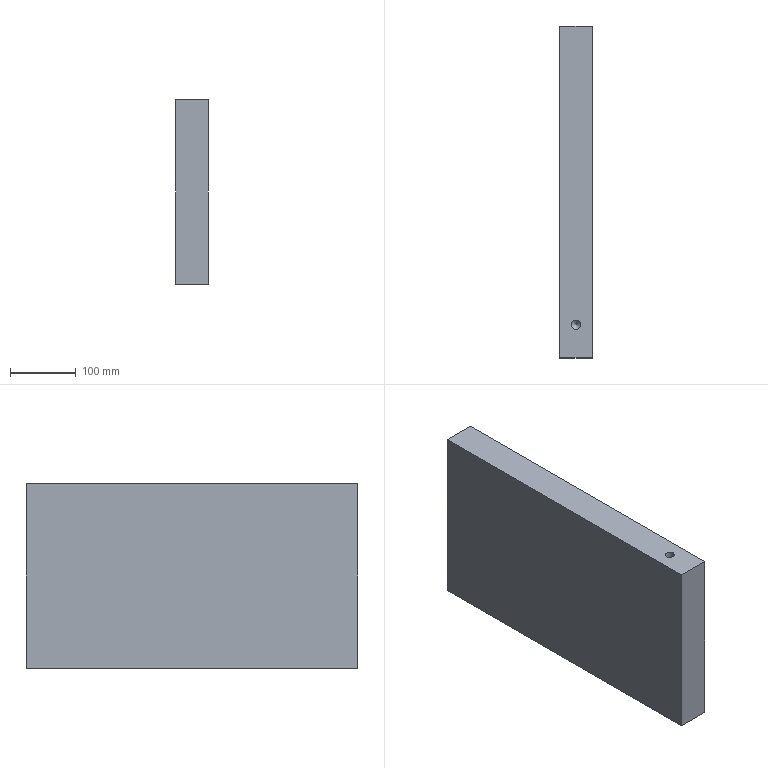Part | NX | features 29 2 | 1 solid | 12 faces | box 50 x 503.5 x 280.5 mm | volume 7043178 mm3 | plane 6 | cylinder 3 | cone 3 | commonest cylinder face diameters 14.1 x3
STEP:
#1=CARTESIAN_POINT('',(3262.05,-622.5,-493.5));
#2=VERTEX_POINT('',#1);
#3=CARTESIAN_POINT('',(3255.,-622.5,-493.5));
#4=DIRECTION('',(0.,0.,1.));
#5=DIRECTION('',(1.,0.,0.));
#6=AXIS2_PLACEMENT_3D('',#3,#4,#5);
#7=CIRCLE('',#6,7.05);
#8=EDGE_CURVE('',#2,#2,#7,.T.);
#9=ORIENTED_EDGE('',*,*,#8,.T.);
#10=EDGE_LOOP('',(#9));
#11=FACE_BOUND('',#10,.T.);
#12=CARTESIAN_POINT('',(3230.,-169.,-493.5));
#13=VERTEX_POINT('',#12);
#14=CARTESIAN_POINT('',(3230.,-672.5,-493.5));
#15=VERTEX_POINT('',#14);
#16=CARTESIAN_POINT('',(3230.,193.,-493.5));
#17=DIRECTION('',(0.,-1.,0.));
#18=VECTOR('',#17,1000.);
#19=LINE('',#16,#18);
#20=EDGE_CURVE('',#13,#15,#19,.T.);
#21=ORIENTED_EDGE('',*,*,#20,.F.);
#22=CARTESIAN_POINT('',(3280.,-169.,-493.5));
#23=VERTEX_POINT('',#22);
#24=CARTESIAN_POINT('',(1945.,-169.,-493.5));
#25=DIRECTION('',(1.,0.,0.));
#26=VECTOR('',#25,1000.);
#27=LINE('',#24,#26);
#28=EDGE_CURVE('',#13,#23,#27,.T.);
#29=ORIENTED_EDGE('',*,*,#28,.T.);
#30=CARTESIAN_POINT('',(3280.,-672.5,-493.5));
#31=VERTEX_POINT('',#30);
#32=CARTESIAN_POINT('',(3280.,193.,-493.5));
#33=DIRECTION('',(0.,1.,0.));
#34=VECTOR('',#33,1000.);
#35=LINE('',#32,#34);
#36=EDGE_CURVE('',#31,#23,#35,.T.);
#37=ORIENTED_EDGE('',*,*,#36,.F.);
#38=CARTESIAN_POINT('',(3620.,-672.5,-493.5));
#39=DIRECTION('',(-1.,0.,0.));
#40=VECTOR('',#39,1000.);
#41=LINE('',#38,#40);
#42=EDGE_CURVE('',#31,#15,#41,.T.);
#43=ORIENTED_EDGE('',*,*,#42,.T.);
#44=EDGE_LOOP('',(#21,#29,#37,#43));
#45=FACE_BOUND('',#44,.T.);
#46=CARTESIAN_POINT('',(3262.05,-242.5,-493.5));
#47=VERTEX_POINT('',#46);
#48=CARTESIAN_POINT('',(3255.,-242.5,-493.5));
#49=DIRECTION('',(0.,0.,1.));
#50=DIRECTION('',(1.,0.,0.));
#51=AXIS2_PLACEMENT_3D('',#48,#49,#50);
#52=CIRCLE('',#51,7.05);
#53=EDGE_CURVE('',#47,#47,#52,.T.);
#54=ORIENTED_EDGE('',*,*,#53,.T.);
#55=EDGE_LOOP('',(#54));
#56=FACE_BOUND('',#55,.T.);
#57=CARTESIAN_POINT('',(1945.,0.,-493.5));
#58=DIRECTION('',(0.,0.,-1.));
#59=DIRECTION('',(1.,0.,0.));
#60=AXIS2_PLACEMENT_3D('',#57,#58,#59);
#61=PLANE('',#60);
#62=ADVANCED_FACE('',(#11,#45,#56),#61,.T.);
#63=CARTESIAN_POINT('',(3280.,-169.,-213.));
#64=VERTEX_POINT('',#63);
#65=CARTESIAN_POINT('',(3280.,-672.5,-213.));
#66=VERTEX_POINT('',#65);
#67=CARTESIAN_POINT('',(3280.,193.,-213.));
#68=DIRECTION('',(0.,-1.,0.));
#69=VECTOR('',#68,1000.);
#70=LINE('',#67,#69);
#71=EDGE_CURVE('',#64,#66,#70,.T.);
#72=ORIENTED_EDGE('',*,*,#71,.F.);
#73=CARTESIAN_POINT('',(3230.,-169.,-213.));
#74=VERTEX_POINT('',#73);
#75=CARTESIAN_POINT('',(1945.,-169.,-213.));
#76=DIRECTION('',(-1.,0.,0.));
#77=VECTOR('',#76,1000.);
#78=LINE('',#75,#77);
#79=EDGE_CURVE('',#64,#74,#78,.T.);
#80=ORIENTED_EDGE('',*,*,#79,.T.);
#81=CARTESIAN_POINT('',(3230.,-672.5,-213.));
#82=VERTEX_POINT('',#81);
#83=CARTESIAN_POINT('',(3230.,193.,-213.));
#84=DIRECTION('',(0.,1.,0.));
#85=VECTOR('',#84,1000.);
#86=LINE('',#83,#85);
#87=EDGE_CURVE('',#82,#74,#86,.T.);
#88=ORIENTED_EDGE('',*,*,#87,.F.);
#89=CARTESIAN_POINT('',(3620.,-672.5,-213.));
#90=DIRECTION('',(1.,0.,0.));
#91=VECTOR('',#90,1000.);
#92=LINE('',#89,#91);
#93=EDGE_CURVE('',#82,#66,#92,.T.);
#94=ORIENTED_EDGE('',*,*,#93,.T.);
#95=EDGE_LOOP('',(#72,#80,#88,#94));
#96=FACE_BOUND('',#95,.T.);
#97=CARTESIAN_POINT('',(3262.05,-622.5,-213.));
#98=VERTEX_POINT('',#97);
#99=CARTESIAN_POINT('',(3255.,-622.5,-213.));
#100=DIRECTION('',(0.,0.,-1.));
#101=DIRECTION('',(1.,0.,0.));
#102=AXIS2_PLACEMENT_3D('',#99,#100,#101);
#103=CIRCLE('',#102,7.05);
#104=EDGE_CURVE('',#98,#98,#103,.T.);
#105=ORIENTED_EDGE('',*,*,#104,.T.);
#106=EDGE_LOOP('',(#105));
#107=FACE_BOUND('',#106,.T.);
#108=CARTESIAN_POINT('',(1945.,0.,-213.));
#109=DIRECTION('',(0.,0.,1.));
#110=DIRECTION('',(-1.,0.,0.));
#111=AXIS2_PLACEMENT_3D('',#108,#109,#110);
#112=PLANE('',#111);
#113=ADVANCED_FACE('',(#96,#107),#112,.T.);
#114=CARTESIAN_POINT('',(3280.,-169.,-205.5));
#115=DIRECTION('',(0.,0.,1.));
#116=VECTOR('',#115,1000.);
#117=LINE('',#114,#116);
#118=EDGE_CURVE('',#23,#64,#117,.T.);
#119=ORIENTED_EDGE('',*,*,#118,.F.);
#120=ORIENTED_EDGE('',*,*,#28,.F.);
#121=CARTESIAN_POINT('',(3230.,-169.,-205.5));
#122=DIRECTION('',(0.,0.,-1.));
#123=VECTOR('',#122,1000.);
#124=LINE('',#121,#123);
#125=EDGE_CURVE('',#74,#13,#124,.T.);
#126=ORIENTED_EDGE('',*,*,#125,.F.);
#127=ORIENTED_EDGE('',*,*,#79,.F.);
#128=EDGE_LOOP('',(#119,#120,#126,#127));
#129=FACE_BOUND('',#128,.T.);
#130=CARTESIAN_POINT('',(2891.,-169.,0.));
#131=DIRECTION('',(0.,1.,0.));
#132=DIRECTION('',(0.,0.,-1.));
#133=AXIS2_PLACEMENT_3D('',#130,#131,#132);
#134=PLANE('',#133);
#135=ADVANCED_FACE('',(#129),#134,.T.);
#136=ORIENTED_EDGE('',*,*,#36,.T.);
#137=ORIENTED_EDGE('',*,*,#118,.T.);
#138=ORIENTED_EDGE('',*,*,#71,.T.);
#139=CARTESIAN_POINT('',(3280.,-672.5,-543.5));
#140=DIRECTION('',(0.,0.,1.));
#141=VECTOR('',#140,1000.);
#142=LINE('',#139,#141);
#143=EDGE_CURVE('',#31,#66,#142,.T.);
#144=ORIENTED_EDGE('',*,*,#143,.F.);
#145=EDGE_LOOP('',(#136,#137,#138,#144));
#146=FACE_BOUND('',#145,.T.);
#147=CARTESIAN_POINT('',(3280.,193.,-205.5));
#148=DIRECTION('',(1.,0.,0.));
#149=DIRECTION('',(0.,0.,-1.));
#150=AXIS2_PLACEMENT_3D('',#147,#148,#149);
#151=PLANE('',#150);
#152=ADVANCED_FACE('',(#146),#151,.T.);
#153=ORIENTED_EDGE('',*,*,#87,.T.);
#154=ORIENTED_EDGE('',*,*,#125,.T.);
#155=ORIENTED_EDGE('',*,*,#20,.T.);
#156=CARTESIAN_POINT('',(3230.,-672.5,-113.));
#157=DIRECTION('',(0.,0.,1.));
#158=VECTOR('',#157,1000.);
#159=LINE('',#156,#158);
#160=EDGE_CURVE('',#15,#82,#159,.T.);
#161=ORIENTED_EDGE('',*,*,#160,.T.);
#162=EDGE_LOOP('',(#153,#154,#155,#161));
#163=FACE_BOUND('',#162,.T.);
#164=CARTESIAN_POINT('',(3230.,193.,-205.5));
#165=DIRECTION('',(-1.,0.,0.));
#166=DIRECTION('',(0.,0.,1.));
#167=AXIS2_PLACEMENT_3D('',#164,#165,#166);
#168=PLANE('',#167);
#169=ADVANCED_FACE('',(#163),#168,.T.);
#170=ORIENTED_EDGE('',*,*,#42,.F.);
#171=ORIENTED_EDGE('',*,*,#143,.T.);
#172=ORIENTED_EDGE('',*,*,#93,.F.);
#173=ORIENTED_EDGE('',*,*,#160,.F.);
#174=EDGE_LOOP('',(#170,#171,#172,#173));
#175=FACE_BOUND('',#174,.T.);
#176=CARTESIAN_POINT('',(3620.,-672.5,-113.));
#177=DIRECTION('',(0.,1.,0.));
#178=DIRECTION('',(1.,0.,0.));
#179=AXIS2_PLACEMENT_3D('',#176,#177,#178);
#180=PLANE('',#179);
#181=ADVANCED_FACE('',(#175),#180,.F.);
#182=CARTESIAN_POINT('',(3247.95,-622.5,-249.95));
#183=VERTEX_POINT('',#182);
#184=CARTESIAN_POINT('',(3255.,-622.5,-249.95));
#185=DIRECTION('',(0.,0.,-1.));
#186=DIRECTION('',(-1.,0.,0.));
#187=AXIS2_PLACEMENT_3D('',#184,#185,#186);
#188=CIRCLE('',#187,7.05);
#189=EDGE_CURVE('',#183,#183,#188,.T.);
#190=ORIENTED_EDGE('',*,*,#189,.T.);
#191=EDGE_LOOP('',(#190));
#192=FACE_BOUND('',#191,.T.);
#193=ORIENTED_EDGE('',*,*,#104,.F.);
#194=EDGE_LOOP('',(#193));
#195=FACE_BOUND('',#194,.T.);
#196=CARTESIAN_POINT('',(3255.,-622.5,-213.));
#197=DIRECTION('',(0.,0.,-1.));
#198=DIRECTION('',(-1.,0.,0.));
#199=AXIS2_PLACEMENT_3D('',#196,#197,#198);
#200=CYLINDRICAL_SURFACE('',#199,7.05);
#201=ADVANCED_FACE('',(#192,#195),#200,.F.);
#202=CARTESIAN_POINT('',(3255.,-622.5,-257.));
#203=VERTEX_POINT('',#202);
#204=VERTEX_LOOP('',#203);
#205=FACE_BOUND('',#204,.T.);
#206=ORIENTED_EDGE('',*,*,#189,.F.);
#207=EDGE_LOOP('',(#206));
#208=FACE_BOUND('',#207,.T.);
#209=CARTESIAN_POINT('',(3255.,-622.5,-249.95));
#210=DIRECTION('',(0.,0.,1.));
#211=DIRECTION('',(-1.,0.,0.));
#212=AXIS2_PLACEMENT_3D('',#209,#210,#211);
#213=CONICAL_SURFACE('',#212,7.05,0.7854);
#214=ADVANCED_FACE('',(#205,#208),#213,.F.);
#215=CARTESIAN_POINT('',(3262.05,-622.5,-456.55));
#216=VERTEX_POINT('',#215);
#217=CARTESIAN_POINT('',(3255.,-622.5,-456.55));
#218=DIRECTION('',(0.,0.,1.));
#219=DIRECTION('',(1.,0.,0.));
#220=AXIS2_PLACEMENT_3D('',#217,#218,#219);
#221=CIRCLE('',#220,7.05);
#222=EDGE_CURVE('',#216,#216,#221,.T.);
#223=ORIENTED_EDGE('',*,*,#222,.T.);
#224=EDGE_LOOP('',(#223));
#225=FACE_BOUND('',#224,.T.);
#226=ORIENTED_EDGE('',*,*,#8,.F.);
#227=EDGE_LOOP('',(#226));
#228=FACE_BOUND('',#227,.T.);
#229=CARTESIAN_POINT('',(3255.,-622.5,-493.5));
#230=DIRECTION('',(0.,0.,1.));
#231=DIRECTION('',(-1.,0.,0.));
#232=AXIS2_PLACEMENT_3D('',#229,#230,#231);
#233=CYLINDRICAL_SURFACE('',#232,7.05);
#234=ADVANCED_FACE('',(#225,#228),#233,.F.);
#235=CARTESIAN_POINT('',(3255.,-622.5,-449.5));
#236=VERTEX_POINT('',#235);
#237=VERTEX_LOOP('',#236);
#238=FACE_BOUND('',#237,.T.);
#239=ORIENTED_EDGE('',*,*,#222,.F.);
#240=EDGE_LOOP('',(#239));
#241=FACE_BOUND('',#240,.T.);
#242=CARTESIAN_POINT('',(3255.,-622.5,-456.55));
#243=DIRECTION('',(0.,0.,-1.));
#244=DIRECTION('',(1.,0.,0.));
#245=AXIS2_PLACEMENT_3D('',#242,#243,#244);
#246=CONICAL_SURFACE('',#245,7.05,0.7854);
#247=ADVANCED_FACE('',(#238,#241),#246,.F.);
#248=CARTESIAN_POINT('',(3262.05,-242.5,-456.55));
#249=VERTEX_POINT('',#248);
#250=CARTESIAN_POINT('',(3255.,-242.5,-456.55));
#251=DIRECTION('',(0.,0.,1.));
#252=DIRECTION('',(1.,0.,0.));
#253=AXIS2_PLACEMENT_3D('',#250,#251,#252);
#254=CIRCLE('',#253,7.05);
#255=EDGE_CURVE('',#249,#249,#254,.T.);
#256=ORIENTED_EDGE('',*,*,#255,.T.);
#257=EDGE_LOOP('',(#256));
#258=FACE_BOUND('',#257,.T.);
#259=ORIENTED_EDGE('',*,*,#53,.F.);
#260=EDGE_LOOP('',(#259));
#261=FACE_BOUND('',#260,.T.);
#262=CARTESIAN_POINT('',(3255.,-242.5,-493.5));
#263=DIRECTION('',(0.,0.,1.));
#264=DIRECTION('',(-1.,0.,0.));
#265=AXIS2_PLACEMENT_3D('',#262,#263,#264);
#266=CYLINDRICAL_SURFACE('',#265,7.05);
#267=ADVANCED_FACE('',(#258,#261),#266,.F.);
#268=CARTESIAN_POINT('',(3255.,-242.5,-449.5));
#269=VERTEX_POINT('',#268);
#270=VERTEX_LOOP('',#269);
#271=FACE_BOUND('',#270,.T.);
#272=ORIENTED_EDGE('',*,*,#255,.F.);
#273=EDGE_LOOP('',(#272));
#274=FACE_BOUND('',#273,.T.);
#275=CARTESIAN_POINT('',(3255.,-242.5,-456.55));
#276=DIRECTION('',(0.,0.,-1.));
#277=DIRECTION('',(1.,0.,0.));
#278=AXIS2_PLACEMENT_3D('',#275,#276,#277);
#279=CONICAL_SURFACE('',#278,7.05,0.7854);
#280=ADVANCED_FACE('',(#271,#274),#279,.F.);
#281=CLOSED_SHELL('',(#62,#113,#135,#152,#169,#181,#201,#214,#234,#247,#267,#280));
#282=MANIFOLD_SOLID_BREP('',#281);
#283=(LENGTH_UNIT()NAMED_UNIT(*)SI_UNIT(.MILLI.,.METRE.));
#284=UNCERTAINTY_MEASURE_WITH_UNIT(LENGTH_MEASURE(0.00001),#283,'','');
#285=(NAMED_UNIT(*)PLANE_ANGLE_UNIT()SI_UNIT($,.RADIAN.));
#286=(NAMED_UNIT(*)SI_UNIT($,.STERADIAN.)SOLID_ANGLE_UNIT());
#287=(GEOMETRIC_REPRESENTATION_CONTEXT(3)GLOBAL_UNCERTAINTY_ASSIGNED_CONTEXT((#284))GLOBAL_UNIT_ASSIGNED_CONTEXT((#283,#285,#286))REPRESENTATION_CONTEXT('',''));
#288=ADVANCED_BREP_SHAPE_REPRESENTATION('',(#282),#287);